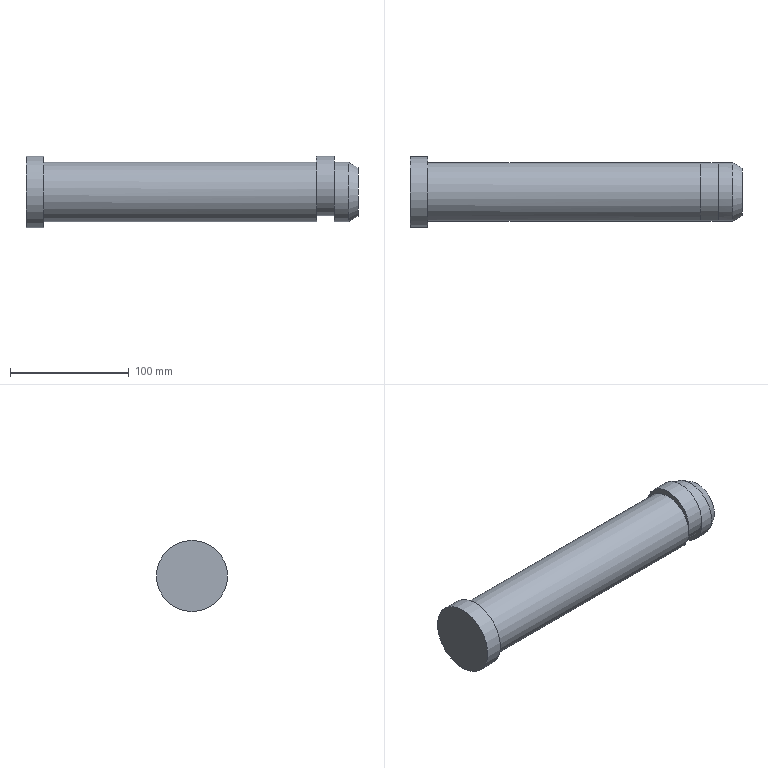Part | NX | features solid 2 | 1 solid | 12 faces | box 280 x 60 x 60 mm | volume 560014 mm3 | plane 7 | cylinder 4 | cone 1 | commonest cylinder face diameters 50 x3 60 x1
STEP:
#1=CARTESIAN_POINT('',(-1065.,-620.,215.));
#2=VERTEX_POINT('',#1);
#3=CARTESIAN_POINT('',(-1065.,-620.,240.));
#4=DIRECTION('',(1.,0.,0.));
#5=DIRECTION('',(0.,0.,-1.));
#6=AXIS2_PLACEMENT_3D('',#3,#4,#5);
#7=CIRCLE('',#6,25.);
#8=EDGE_CURVE('',#2,#2,#7,.F.);
#9=ORIENTED_EDGE('',*,*,#8,.F.);
#10=EDGE_LOOP('',(#9));
#11=FACE_BOUND('',#10,.T.);
#12=CARTESIAN_POINT('',(-835.,-644.875,242.5));
#13=VERTEX_POINT('',#12);
#14=CARTESIAN_POINT('',(-835.,-595.125,242.5));
#15=VERTEX_POINT('',#14);
#16=CARTESIAN_POINT('',(-835.,-620.,240.));
#17=DIRECTION('',(-1.,0.,0.));
#18=DIRECTION('',(0.,1.,0.));
#19=AXIS2_PLACEMENT_3D('',#16,#17,#18);
#20=CIRCLE('',#19,25.);
#21=EDGE_CURVE('',#13,#15,#20,.T.);
#22=ORIENTED_EDGE('',*,*,#21,.T.);
#23=CARTESIAN_POINT('',(-835.,-620.,240.));
#24=DIRECTION('',(-1.,0.,0.));
#25=DIRECTION('',(0.,1.,0.));
#26=AXIS2_PLACEMENT_3D('',#23,#24,#25);
#27=CIRCLE('',#26,25.);
#28=EDGE_CURVE('',#15,#13,#27,.T.);
#29=ORIENTED_EDGE('',*,*,#28,.T.);
#30=EDGE_LOOP('',(#22,#29));
#31=FACE_BOUND('',#30,.T.);
#32=CARTESIAN_POINT('',(-835.,-620.,240.));
#33=DIRECTION('',(-1.,0.,0.));
#34=DIRECTION('',(0.,0.,1.));
#35=AXIS2_PLACEMENT_3D('',#32,#33,#34);
#36=CYLINDRICAL_SURFACE('',#35,25.);
#37=ADVANCED_FACE('',(#11,#31),#36,.T.);
#38=ORIENTED_EDGE('',*,*,#28,.F.);
#39=CARTESIAN_POINT('',(-835.,-620.,245.));
#40=DIRECTION('',(-1.,0.,0.));
#41=DIRECTION('',(0.,1.,0.));
#42=AXIS2_PLACEMENT_3D('',#39,#40,#41);
#43=CIRCLE('',#42,25.);
#44=EDGE_CURVE('',#15,#13,#43,.T.);
#45=ORIENTED_EDGE('',*,*,#44,.T.);
#46=EDGE_LOOP('',(#38,#45));
#47=FACE_BOUND('',#46,.T.);
#48=CARTESIAN_POINT('',(-835.,-620.,240.));
#49=DIRECTION('',(-1.,0.,0.));
#50=DIRECTION('',(0.,0.,1.));
#51=AXIS2_PLACEMENT_3D('',#48,#49,#50);
#52=PLANE('',#51);
#53=ADVANCED_FACE('',(#47),#52,.F.);
#54=CARTESIAN_POINT('',(-1080.,-620.,270.));
#55=VERTEX_POINT('',#54);
#56=CARTESIAN_POINT('',(-1080.,-620.,240.));
#57=DIRECTION('',(-1.,0.,0.));
#58=DIRECTION('',(0.,0.,1.));
#59=AXIS2_PLACEMENT_3D('',#56,#57,#58);
#60=CIRCLE('',#59,30.);
#61=EDGE_CURVE('',#55,#55,#60,.T.);
#62=ORIENTED_EDGE('',*,*,#61,.F.);
#63=EDGE_LOOP('',(#62));
#64=FACE_BOUND('',#63,.T.);
#65=CARTESIAN_POINT('',(-1065.,-620.,270.));
#66=VERTEX_POINT('',#65);
#67=CARTESIAN_POINT('',(-1065.,-620.,240.));
#68=DIRECTION('',(-1.,0.,0.));
#69=DIRECTION('',(0.,0.,1.));
#70=AXIS2_PLACEMENT_3D('',#67,#68,#69);
#71=CIRCLE('',#70,30.);
#72=EDGE_CURVE('',#66,#66,#71,.T.);
#73=ORIENTED_EDGE('',*,*,#72,.T.);
#74=EDGE_LOOP('',(#73));
#75=FACE_BOUND('',#74,.T.);
#76=CARTESIAN_POINT('',(-1065.,-620.,240.));
#77=DIRECTION('',(-1.,0.,0.));
#78=DIRECTION('',(0.,0.,1.));
#79=AXIS2_PLACEMENT_3D('',#76,#77,#78);
#80=CYLINDRICAL_SURFACE('',#79,30.);
#81=ADVANCED_FACE('',(#64,#75),#80,.T.);
#82=ORIENTED_EDGE('',*,*,#72,.F.);
#83=EDGE_LOOP('',(#82));
#84=FACE_BOUND('',#83,.T.);
#85=ORIENTED_EDGE('',*,*,#8,.T.);
#86=EDGE_LOOP('',(#85));
#87=FACE_BOUND('',#86,.T.);
#88=CARTESIAN_POINT('',(-1065.,-620.,240.));
#89=DIRECTION('',(1.,0.,0.));
#90=DIRECTION('',(0.,0.,-1.));
#91=AXIS2_PLACEMENT_3D('',#88,#89,#90);
#92=PLANE('',#91);
#93=ADVANCED_FACE('',(#84,#87),#92,.T.);
#94=ORIENTED_EDGE('',*,*,#61,.T.);
#95=EDGE_LOOP('',(#94));
#96=FACE_BOUND('',#95,.T.);
#97=CARTESIAN_POINT('',(-1080.,-620.,240.));
#98=DIRECTION('',(-1.,0.,0.));
#99=DIRECTION('',(0.,0.,1.));
#100=AXIS2_PLACEMENT_3D('',#97,#98,#99);
#101=PLANE('',#100);
#102=ADVANCED_FACE('',(#96),#101,.T.);
#103=ORIENTED_EDGE('',*,*,#21,.F.);
#104=CARTESIAN_POINT('',(-835.,-620.,245.));
#105=DIRECTION('',(-1.,0.,0.));
#106=DIRECTION('',(0.,1.,0.));
#107=AXIS2_PLACEMENT_3D('',#104,#105,#106);
#108=CIRCLE('',#107,25.);
#109=EDGE_CURVE('',#13,#15,#108,.T.);
#110=ORIENTED_EDGE('',*,*,#109,.T.);
#111=EDGE_LOOP('',(#103,#110));
#112=FACE_BOUND('',#111,.T.);
#113=CARTESIAN_POINT('',(-835.,-620.,245.));
#114=DIRECTION('',(-1.,0.,0.));
#115=DIRECTION('',(0.,0.,1.));
#116=AXIS2_PLACEMENT_3D('',#113,#114,#115);
#117=PLANE('',#116);
#118=ADVANCED_FACE('',(#112),#117,.T.);
#119=CARTESIAN_POINT('',(-820.,-595.125,242.5));
#120=VERTEX_POINT('',#119);
#121=CARTESIAN_POINT('',(-820.,-644.875,242.5));
#122=VERTEX_POINT('',#121);
#123=CARTESIAN_POINT('',(-820.,-620.,245.));
#124=DIRECTION('',(-1.,0.,0.));
#125=DIRECTION('',(0.,1.,0.));
#126=AXIS2_PLACEMENT_3D('',#123,#124,#125);
#127=CIRCLE('',#126,25.);
#128=EDGE_CURVE('',#120,#122,#127,.T.);
#129=ORIENTED_EDGE('',*,*,#128,.T.);
#130=CARTESIAN_POINT('',(-820.,-620.,245.));
#131=DIRECTION('',(-1.,0.,0.));
#132=DIRECTION('',(0.,1.,0.));
#133=AXIS2_PLACEMENT_3D('',#130,#131,#132);
#134=CIRCLE('',#133,25.);
#135=EDGE_CURVE('',#122,#120,#134,.T.);
#136=ORIENTED_EDGE('',*,*,#135,.T.);
#137=EDGE_LOOP('',(#129,#136));
#138=FACE_BOUND('',#137,.T.);
#139=ORIENTED_EDGE('',*,*,#44,.F.);
#140=ORIENTED_EDGE('',*,*,#109,.F.);
#141=EDGE_LOOP('',(#139,#140));
#142=FACE_BOUND('',#141,.T.);
#143=CARTESIAN_POINT('',(-820.,-620.,245.));
#144=DIRECTION('',(-1.,0.,0.));
#145=DIRECTION('',(0.,0.,1.));
#146=AXIS2_PLACEMENT_3D('',#143,#144,#145);
#147=CYLINDRICAL_SURFACE('',#146,25.);
#148=ADVANCED_FACE('',(#138,#142),#147,.T.);
#149=ORIENTED_EDGE('',*,*,#135,.F.);
#150=CARTESIAN_POINT('',(-820.,-620.,240.));
#151=DIRECTION('',(-1.,0.,0.));
#152=DIRECTION('',(0.,1.,0.));
#153=AXIS2_PLACEMENT_3D('',#150,#151,#152);
#154=CIRCLE('',#153,25.);
#155=EDGE_CURVE('',#122,#120,#154,.T.);
#156=ORIENTED_EDGE('',*,*,#155,.T.);
#157=EDGE_LOOP('',(#149,#156));
#158=FACE_BOUND('',#157,.T.);
#159=CARTESIAN_POINT('',(-820.,-620.,245.));
#160=DIRECTION('',(-1.,0.,0.));
#161=DIRECTION('',(0.,0.,1.));
#162=AXIS2_PLACEMENT_3D('',#159,#160,#161);
#163=PLANE('',#162);
#164=ADVANCED_FACE('',(#158),#163,.F.);
#165=ORIENTED_EDGE('',*,*,#128,.F.);
#166=CARTESIAN_POINT('',(-820.,-620.,240.));
#167=DIRECTION('',(-1.,0.,0.));
#168=DIRECTION('',(0.,1.,0.));
#169=AXIS2_PLACEMENT_3D('',#166,#167,#168);
#170=CIRCLE('',#169,25.);
#171=EDGE_CURVE('',#120,#122,#170,.T.);
#172=ORIENTED_EDGE('',*,*,#171,.T.);
#173=EDGE_LOOP('',(#165,#172));
#174=FACE_BOUND('',#173,.T.);
#175=CARTESIAN_POINT('',(-820.,-620.,240.));
#176=DIRECTION('',(-1.,0.,0.));
#177=DIRECTION('',(0.,0.,1.));
#178=AXIS2_PLACEMENT_3D('',#175,#176,#177);
#179=PLANE('',#178);
#180=ADVANCED_FACE('',(#174),#179,.T.);
#181=CARTESIAN_POINT('',(-808.,-620.,265.));
#182=VERTEX_POINT('',#181);
#183=CARTESIAN_POINT('',(-808.,-620.,240.));
#184=DIRECTION('',(-1.,0.,0.));
#185=DIRECTION('',(0.,0.,1.));
#186=AXIS2_PLACEMENT_3D('',#183,#184,#185);
#187=CIRCLE('',#186,25.);
#188=EDGE_CURVE('',#182,#182,#187,.T.);
#189=ORIENTED_EDGE('',*,*,#188,.T.);
#190=EDGE_LOOP('',(#189));
#191=FACE_BOUND('',#190,.T.);
#192=ORIENTED_EDGE('',*,*,#155,.F.);
#193=ORIENTED_EDGE('',*,*,#171,.F.);
#194=EDGE_LOOP('',(#192,#193));
#195=FACE_BOUND('',#194,.T.);
#196=CARTESIAN_POINT('',(-800.,-620.,240.));
#197=DIRECTION('',(-1.,0.,0.));
#198=DIRECTION('',(0.,0.,1.));
#199=AXIS2_PLACEMENT_3D('',#196,#197,#198);
#200=CYLINDRICAL_SURFACE('',#199,25.);
#201=ADVANCED_FACE('',(#191,#195),#200,.T.);
#202=CARTESIAN_POINT('',(-800.,-620.,260.381));
#203=VERTEX_POINT('',#202);
#204=CARTESIAN_POINT('',(-800.,-620.,240.));
#205=DIRECTION('',(-1.,0.,0.));
#206=DIRECTION('',(0.,0.,1.));
#207=AXIS2_PLACEMENT_3D('',#204,#205,#206);
#208=CIRCLE('',#207,20.381);
#209=EDGE_CURVE('',#203,#203,#208,.F.);
#210=ORIENTED_EDGE('',*,*,#209,.T.);
#211=EDGE_LOOP('',(#210));
#212=FACE_BOUND('',#211,.T.);
#213=CARTESIAN_POINT('',(-800.,-620.,240.));
#214=DIRECTION('',(-1.,0.,0.));
#215=DIRECTION('',(0.,0.,1.));
#216=AXIS2_PLACEMENT_3D('',#213,#214,#215);
#217=PLANE('',#216);
#218=ADVANCED_FACE('',(#212),#217,.F.);
#219=ORIENTED_EDGE('',*,*,#209,.F.);
#220=EDGE_LOOP('',(#219));
#221=FACE_BOUND('',#220,.T.);
#222=ORIENTED_EDGE('',*,*,#188,.F.);
#223=EDGE_LOOP('',(#222));
#224=FACE_BOUND('',#223,.T.);
#225=CARTESIAN_POINT('',(-808.,-620.,240.));
#226=DIRECTION('',(-1.,0.,0.));
#227=DIRECTION('',(0.,0.,1.));
#228=AXIS2_PLACEMENT_3D('',#225,#226,#227);
#229=CONICAL_SURFACE('',#228,25.,0.5236);
#230=ADVANCED_FACE('',(#221,#224),#229,.T.);
#231=CLOSED_SHELL('',(#37,#53,#81,#93,#102,#118,#148,#164,#180,#201,#218,#230));
#232=MANIFOLD_SOLID_BREP('',#231);
#233=(LENGTH_UNIT()NAMED_UNIT(*)SI_UNIT(.MILLI.,.METRE.));
#234=UNCERTAINTY_MEASURE_WITH_UNIT(LENGTH_MEASURE(0.00001),#233,'','');
#235=(NAMED_UNIT(*)PLANE_ANGLE_UNIT()SI_UNIT($,.RADIAN.));
#236=(NAMED_UNIT(*)SI_UNIT($,.STERADIAN.)SOLID_ANGLE_UNIT());
#237=(GEOMETRIC_REPRESENTATION_CONTEXT(3)GLOBAL_UNCERTAINTY_ASSIGNED_CONTEXT((#234))GLOBAL_UNIT_ASSIGNED_CONTEXT((#233,#235,#236))REPRESENTATION_CONTEXT('',''));
#238=ADVANCED_BREP_SHAPE_REPRESENTATION('',(#232),#237);